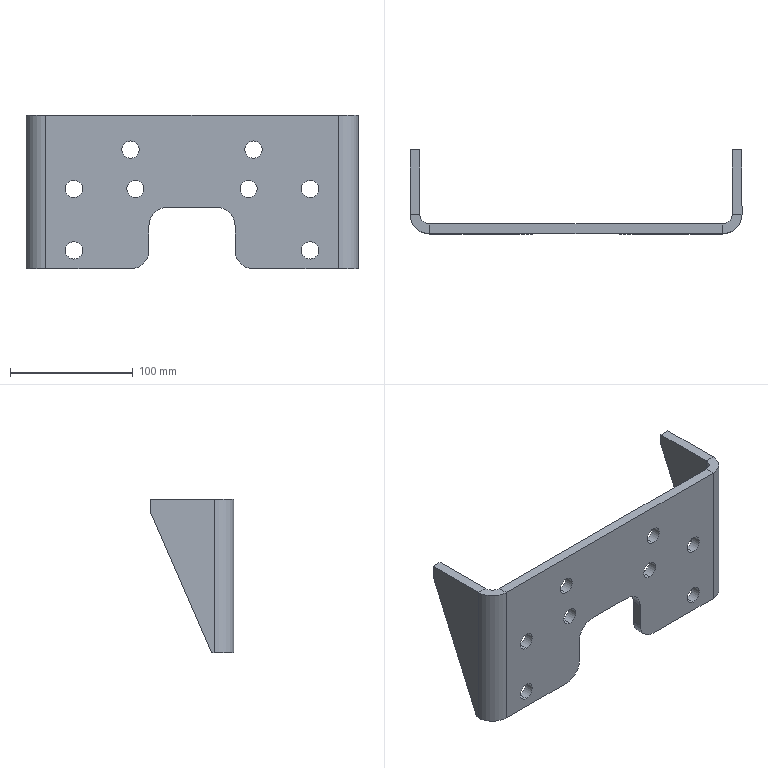Part | SolidWorks | features Extrusion 1, FlatPattern 1, SM3dBend 1, SheetMetal 1, SolidToSheetMetal 1 | 1 solid | 48 faces | box 270 x 68.15 x 125 mm | volume 296148 mm3 | cylinder 24 | plane 24 | commonest cylinder face diameters 14 x16 30 x4 16 x2 32 x2
STEP:
#1=CARTESIAN_POINT('',(96.,8.,-117.));
#2=VERTEX_POINT('',#1);
#3=CARTESIAN_POINT('',(96.,8.,-103.));
#4=VERTEX_POINT('',#3);
#5=CARTESIAN_POINT('',(96.,8.,-110.));
#6=DIRECTION('',(0.,1.,0.));
#7=DIRECTION('',(0.,0.,-1.));
#8=AXIS2_PLACEMENT_3D('',#5,#6,#7);
#9=CIRCLE('',#8,7.);
#10=EDGE_CURVE('',#2,#4,#9,.T.);
#11=ORIENTED_EDGE('',*,*,#10,.T.);
#12=CARTESIAN_POINT('',(96.,0.,-103.));
#13=VERTEX_POINT('',#12);
#14=CARTESIAN_POINT('',(96.,8.,-103.));
#15=DIRECTION('',(0.,-1.,0.));
#16=VECTOR('',#15,1000.);
#17=LINE('',#14,#16);
#18=EDGE_CURVE('',#4,#13,#17,.T.);
#19=ORIENTED_EDGE('',*,*,#18,.T.);
#20=CARTESIAN_POINT('',(96.,0.,-117.));
#21=VERTEX_POINT('',#20);
#22=CARTESIAN_POINT('',(96.,0.,-110.));
#23=DIRECTION('',(0.,1.,0.));
#24=DIRECTION('',(0.,0.,1.));
#25=AXIS2_PLACEMENT_3D('',#22,#23,#24);
#26=CIRCLE('',#25,7.);
#27=EDGE_CURVE('',#21,#13,#26,.T.);
#28=ORIENTED_EDGE('',*,*,#27,.F.);
#29=CARTESIAN_POINT('',(96.,8.,-117.));
#30=DIRECTION('',(0.,-1.,0.));
#31=VECTOR('',#30,1000.);
#32=LINE('',#29,#31);
#33=EDGE_CURVE('',#2,#21,#32,.T.);
#34=ORIENTED_EDGE('',*,*,#33,.F.);
#35=EDGE_LOOP('',(#11,#19,#28,#34));
#36=FACE_OUTER_BOUND('',#35,.T.);
#37=CARTESIAN_POINT('',(96.,8.,-110.));
#38=DIRECTION('',(0.,-1.,0.));
#39=DIRECTION('',(0.,0.,-1.));
#40=AXIS2_PLACEMENT_3D('',#37,#38,#39);
#41=CYLINDRICAL_SURFACE('',#40,7.);
#42=ADVANCED_FACE('',(#36),#41,.F.);
#43=CARTESIAN_POINT('',(96.,8.,-67.));
#44=VERTEX_POINT('',#43);
#45=CARTESIAN_POINT('',(96.,8.,-53.));
#46=VERTEX_POINT('',#45);
#47=CARTESIAN_POINT('',(96.,8.,-60.));
#48=DIRECTION('',(0.,1.,0.));
#49=DIRECTION('',(0.,0.,-1.));
#50=AXIS2_PLACEMENT_3D('',#47,#48,#49);
#51=CIRCLE('',#50,7.);
#52=EDGE_CURVE('',#44,#46,#51,.T.);
#53=ORIENTED_EDGE('',*,*,#52,.T.);
#54=CARTESIAN_POINT('',(96.,0.,-53.));
#55=VERTEX_POINT('',#54);
#56=CARTESIAN_POINT('',(96.,8.,-53.));
#57=DIRECTION('',(0.,-1.,0.));
#58=VECTOR('',#57,1000.);
#59=LINE('',#56,#58);
#60=EDGE_CURVE('',#46,#55,#59,.T.);
#61=ORIENTED_EDGE('',*,*,#60,.T.);
#62=CARTESIAN_POINT('',(96.,0.,-67.));
#63=VERTEX_POINT('',#62);
#64=CARTESIAN_POINT('',(96.,0.,-60.));
#65=DIRECTION('',(0.,1.,0.));
#66=DIRECTION('',(0.,0.,1.));
#67=AXIS2_PLACEMENT_3D('',#64,#65,#66);
#68=CIRCLE('',#67,7.);
#69=EDGE_CURVE('',#63,#55,#68,.T.);
#70=ORIENTED_EDGE('',*,*,#69,.F.);
#71=CARTESIAN_POINT('',(96.,8.,-67.));
#72=DIRECTION('',(0.,-1.,0.));
#73=VECTOR('',#72,1000.);
#74=LINE('',#71,#73);
#75=EDGE_CURVE('',#44,#63,#74,.T.);
#76=ORIENTED_EDGE('',*,*,#75,.F.);
#77=EDGE_LOOP('',(#53,#61,#70,#76));
#78=FACE_OUTER_BOUND('',#77,.T.);
#79=CARTESIAN_POINT('',(96.,8.,-60.));
#80=DIRECTION('',(0.,-1.,0.));
#81=DIRECTION('',(0.,0.,-1.));
#82=AXIS2_PLACEMENT_3D('',#79,#80,#81);
#83=CYLINDRICAL_SURFACE('',#82,7.);
#84=ADVANCED_FACE('',(#78),#83,.F.);
#85=CARTESIAN_POINT('',(46.,8.,-67.));
#86=VERTEX_POINT('',#85);
#87=CARTESIAN_POINT('',(46.,8.,-53.));
#88=VERTEX_POINT('',#87);
#89=CARTESIAN_POINT('',(46.,8.,-60.));
#90=DIRECTION('',(0.,1.,0.));
#91=DIRECTION('',(0.,0.,-1.));
#92=AXIS2_PLACEMENT_3D('',#89,#90,#91);
#93=CIRCLE('',#92,7.);
#94=EDGE_CURVE('',#86,#88,#93,.T.);
#95=ORIENTED_EDGE('',*,*,#94,.T.);
#96=CARTESIAN_POINT('',(46.,0.,-53.));
#97=VERTEX_POINT('',#96);
#98=CARTESIAN_POINT('',(46.,8.,-53.));
#99=DIRECTION('',(0.,-1.,0.));
#100=VECTOR('',#99,1000.);
#101=LINE('',#98,#100);
#102=EDGE_CURVE('',#88,#97,#101,.T.);
#103=ORIENTED_EDGE('',*,*,#102,.T.);
#104=CARTESIAN_POINT('',(46.,0.,-67.));
#105=VERTEX_POINT('',#104);
#106=CARTESIAN_POINT('',(46.,0.,-60.));
#107=DIRECTION('',(0.,1.,0.));
#108=DIRECTION('',(0.,0.,1.));
#109=AXIS2_PLACEMENT_3D('',#106,#107,#108);
#110=CIRCLE('',#109,7.);
#111=EDGE_CURVE('',#105,#97,#110,.T.);
#112=ORIENTED_EDGE('',*,*,#111,.F.);
#113=CARTESIAN_POINT('',(46.,8.,-67.));
#114=DIRECTION('',(0.,-1.,0.));
#115=VECTOR('',#114,1000.);
#116=LINE('',#113,#115);
#117=EDGE_CURVE('',#86,#105,#116,.T.);
#118=ORIENTED_EDGE('',*,*,#117,.F.);
#119=EDGE_LOOP('',(#95,#103,#112,#118));
#120=FACE_OUTER_BOUND('',#119,.T.);
#121=CARTESIAN_POINT('',(46.,8.,-60.));
#122=DIRECTION('',(0.,-1.,0.));
#123=DIRECTION('',(0.,0.,-1.));
#124=AXIS2_PLACEMENT_3D('',#121,#122,#123);
#125=CYLINDRICAL_SURFACE('',#124,7.);
#126=ADVANCED_FACE('',(#120),#125,.F.);
#127=CARTESIAN_POINT('',(50.,8.,-35.));
#128=VERTEX_POINT('',#127);
#129=CARTESIAN_POINT('',(50.,8.,-21.));
#130=VERTEX_POINT('',#129);
#131=CARTESIAN_POINT('',(50.,8.,-28.));
#132=DIRECTION('',(0.,1.,0.));
#133=DIRECTION('',(0.,0.,-1.));
#134=AXIS2_PLACEMENT_3D('',#131,#132,#133);
#135=CIRCLE('',#134,7.);
#136=EDGE_CURVE('',#128,#130,#135,.T.);
#137=ORIENTED_EDGE('',*,*,#136,.T.);
#138=CARTESIAN_POINT('',(50.,0.,-21.));
#139=VERTEX_POINT('',#138);
#140=CARTESIAN_POINT('',(50.,8.,-21.));
#141=DIRECTION('',(0.,-1.,0.));
#142=VECTOR('',#141,1000.);
#143=LINE('',#140,#142);
#144=EDGE_CURVE('',#130,#139,#143,.T.);
#145=ORIENTED_EDGE('',*,*,#144,.T.);
#146=CARTESIAN_POINT('',(50.,0.,-35.));
#147=VERTEX_POINT('',#146);
#148=CARTESIAN_POINT('',(50.,0.,-28.));
#149=DIRECTION('',(0.,1.,0.));
#150=DIRECTION('',(0.,0.,1.));
#151=AXIS2_PLACEMENT_3D('',#148,#149,#150);
#152=CIRCLE('',#151,7.);
#153=EDGE_CURVE('',#147,#139,#152,.T.);
#154=ORIENTED_EDGE('',*,*,#153,.F.);
#155=CARTESIAN_POINT('',(50.,8.,-35.));
#156=DIRECTION('',(0.,-1.,0.));
#157=VECTOR('',#156,1000.);
#158=LINE('',#155,#157);
#159=EDGE_CURVE('',#128,#147,#158,.T.);
#160=ORIENTED_EDGE('',*,*,#159,.F.);
#161=EDGE_LOOP('',(#137,#145,#154,#160));
#162=FACE_OUTER_BOUND('',#161,.T.);
#163=CARTESIAN_POINT('',(50.,8.,-28.));
#164=DIRECTION('',(0.,-1.,0.));
#165=DIRECTION('',(0.,0.,-1.));
#166=AXIS2_PLACEMENT_3D('',#163,#164,#165);
#167=CYLINDRICAL_SURFACE('',#166,7.);
#168=ADVANCED_FACE('',(#162),#167,.F.);
#169=CARTESIAN_POINT('',(-50.,8.,-35.));
#170=VERTEX_POINT('',#169);
#171=CARTESIAN_POINT('',(-50.,8.,-21.));
#172=VERTEX_POINT('',#171);
#173=CARTESIAN_POINT('',(-50.,8.,-28.));
#174=DIRECTION('',(0.,1.,0.));
#175=DIRECTION('',(0.,0.,1.));
#176=AXIS2_PLACEMENT_3D('',#173,#174,#175);
#177=CIRCLE('',#176,7.);
#178=EDGE_CURVE('',#170,#172,#177,.T.);
#179=ORIENTED_EDGE('',*,*,#178,.T.);
#180=CARTESIAN_POINT('',(-50.,0.,-21.));
#181=VERTEX_POINT('',#180);
#182=CARTESIAN_POINT('',(-50.,8.,-21.));
#183=DIRECTION('',(0.,-1.,0.));
#184=VECTOR('',#183,1000.);
#185=LINE('',#182,#184);
#186=EDGE_CURVE('',#172,#181,#185,.T.);
#187=ORIENTED_EDGE('',*,*,#186,.T.);
#188=CARTESIAN_POINT('',(-50.,0.,-35.));
#189=VERTEX_POINT('',#188);
#190=CARTESIAN_POINT('',(-50.,0.,-28.));
#191=DIRECTION('',(0.,1.,0.));
#192=DIRECTION('',(0.,0.,1.));
#193=AXIS2_PLACEMENT_3D('',#190,#191,#192);
#194=CIRCLE('',#193,7.);
#195=EDGE_CURVE('',#189,#181,#194,.T.);
#196=ORIENTED_EDGE('',*,*,#195,.F.);
#197=CARTESIAN_POINT('',(-50.,8.,-35.));
#198=DIRECTION('',(0.,-1.,0.));
#199=VECTOR('',#198,1000.);
#200=LINE('',#197,#199);
#201=EDGE_CURVE('',#170,#189,#200,.T.);
#202=ORIENTED_EDGE('',*,*,#201,.F.);
#203=EDGE_LOOP('',(#179,#187,#196,#202));
#204=FACE_OUTER_BOUND('',#203,.T.);
#205=CARTESIAN_POINT('',(-50.,8.,-28.));
#206=DIRECTION('',(0.,-1.,0.));
#207=DIRECTION('',(0.,0.,-1.));
#208=AXIS2_PLACEMENT_3D('',#205,#206,#207);
#209=CYLINDRICAL_SURFACE('',#208,7.);
#210=ADVANCED_FACE('',(#204),#209,.F.);
#211=CARTESIAN_POINT('',(-46.,8.,-67.));
#212=VERTEX_POINT('',#211);
#213=CARTESIAN_POINT('',(-46.,8.,-53.));
#214=VERTEX_POINT('',#213);
#215=CARTESIAN_POINT('',(-46.,8.,-60.));
#216=DIRECTION('',(0.,1.,0.));
#217=DIRECTION('',(0.,0.,1.));
#218=AXIS2_PLACEMENT_3D('',#215,#216,#217);
#219=CIRCLE('',#218,7.);
#220=EDGE_CURVE('',#212,#214,#219,.T.);
#221=ORIENTED_EDGE('',*,*,#220,.T.);
#222=CARTESIAN_POINT('',(-46.,0.,-53.));
#223=VERTEX_POINT('',#222);
#224=CARTESIAN_POINT('',(-46.,8.,-53.));
#225=DIRECTION('',(0.,-1.,0.));
#226=VECTOR('',#225,1000.);
#227=LINE('',#224,#226);
#228=EDGE_CURVE('',#214,#223,#227,.T.);
#229=ORIENTED_EDGE('',*,*,#228,.T.);
#230=CARTESIAN_POINT('',(-46.,0.,-67.));
#231=VERTEX_POINT('',#230);
#232=CARTESIAN_POINT('',(-46.,0.,-60.));
#233=DIRECTION('',(0.,1.,0.));
#234=DIRECTION('',(0.,0.,1.));
#235=AXIS2_PLACEMENT_3D('',#232,#233,#234);
#236=CIRCLE('',#235,7.);
#237=EDGE_CURVE('',#231,#223,#236,.T.);
#238=ORIENTED_EDGE('',*,*,#237,.F.);
#239=CARTESIAN_POINT('',(-46.,8.,-67.));
#240=DIRECTION('',(0.,-1.,0.));
#241=VECTOR('',#240,1000.);
#242=LINE('',#239,#241);
#243=EDGE_CURVE('',#212,#231,#242,.T.);
#244=ORIENTED_EDGE('',*,*,#243,.F.);
#245=EDGE_LOOP('',(#221,#229,#238,#244));
#246=FACE_OUTER_BOUND('',#245,.T.);
#247=CARTESIAN_POINT('',(-46.,8.,-60.));
#248=DIRECTION('',(0.,-1.,0.));
#249=DIRECTION('',(0.,0.,-1.));
#250=AXIS2_PLACEMENT_3D('',#247,#248,#249);
#251=CYLINDRICAL_SURFACE('',#250,7.);
#252=ADVANCED_FACE('',(#246),#251,.F.);
#253=CARTESIAN_POINT('',(-96.,8.,-67.));
#254=VERTEX_POINT('',#253);
#255=CARTESIAN_POINT('',(-96.,8.,-53.));
#256=VERTEX_POINT('',#255);
#257=CARTESIAN_POINT('',(-96.,8.,-60.));
#258=DIRECTION('',(0.,1.,0.));
#259=DIRECTION('',(0.,0.,1.));
#260=AXIS2_PLACEMENT_3D('',#257,#258,#259);
#261=CIRCLE('',#260,7.);
#262=EDGE_CURVE('',#254,#256,#261,.T.);
#263=ORIENTED_EDGE('',*,*,#262,.T.);
#264=CARTESIAN_POINT('',(-96.,0.,-53.));
#265=VERTEX_POINT('',#264);
#266=CARTESIAN_POINT('',(-96.,8.,-53.));
#267=DIRECTION('',(0.,-1.,0.));
#268=VECTOR('',#267,1000.);
#269=LINE('',#266,#268);
#270=EDGE_CURVE('',#256,#265,#269,.T.);
#271=ORIENTED_EDGE('',*,*,#270,.T.);
#272=CARTESIAN_POINT('',(-96.,0.,-67.));
#273=VERTEX_POINT('',#272);
#274=CARTESIAN_POINT('',(-96.,0.,-60.));
#275=DIRECTION('',(0.,1.,0.));
#276=DIRECTION('',(0.,0.,1.));
#277=AXIS2_PLACEMENT_3D('',#274,#275,#276);
#278=CIRCLE('',#277,7.);
#279=EDGE_CURVE('',#273,#265,#278,.T.);
#280=ORIENTED_EDGE('',*,*,#279,.F.);
#281=CARTESIAN_POINT('',(-96.,8.,-67.));
#282=DIRECTION('',(0.,-1.,0.));
#283=VECTOR('',#282,1000.);
#284=LINE('',#281,#283);
#285=EDGE_CURVE('',#254,#273,#284,.T.);
#286=ORIENTED_EDGE('',*,*,#285,.F.);
#287=EDGE_LOOP('',(#263,#271,#280,#286));
#288=FACE_OUTER_BOUND('',#287,.T.);
#289=CARTESIAN_POINT('',(-96.,8.,-60.));
#290=DIRECTION('',(0.,-1.,0.));
#291=DIRECTION('',(0.,0.,-1.));
#292=AXIS2_PLACEMENT_3D('',#289,#290,#291);
#293=CYLINDRICAL_SURFACE('',#292,7.);
#294=ADVANCED_FACE('',(#288),#293,.F.);
#295=CARTESIAN_POINT('',(-96.,8.,-117.));
#296=VERTEX_POINT('',#295);
#297=CARTESIAN_POINT('',(-96.,8.,-103.));
#298=VERTEX_POINT('',#297);
#299=CARTESIAN_POINT('',(-96.,8.,-110.));
#300=DIRECTION('',(0.,1.,0.));
#301=DIRECTION('',(0.,0.,1.));
#302=AXIS2_PLACEMENT_3D('',#299,#300,#301);
#303=CIRCLE('',#302,7.);
#304=EDGE_CURVE('',#296,#298,#303,.T.);
#305=ORIENTED_EDGE('',*,*,#304,.T.);
#306=CARTESIAN_POINT('',(-96.,0.,-103.));
#307=VERTEX_POINT('',#306);
#308=CARTESIAN_POINT('',(-96.,8.,-103.));
#309=DIRECTION('',(0.,-1.,0.));
#310=VECTOR('',#309,1000.);
#311=LINE('',#308,#310);
#312=EDGE_CURVE('',#298,#307,#311,.T.);
#313=ORIENTED_EDGE('',*,*,#312,.T.);
#314=CARTESIAN_POINT('',(-96.,0.,-117.));
#315=VERTEX_POINT('',#314);
#316=CARTESIAN_POINT('',(-96.,0.,-110.));
#317=DIRECTION('',(0.,1.,0.));
#318=DIRECTION('',(0.,0.,1.));
#319=AXIS2_PLACEMENT_3D('',#316,#317,#318);
#320=CIRCLE('',#319,7.);
#321=EDGE_CURVE('',#315,#307,#320,.T.);
#322=ORIENTED_EDGE('',*,*,#321,.F.);
#323=CARTESIAN_POINT('',(-96.,8.,-117.));
#324=DIRECTION('',(0.,-1.,0.));
#325=VECTOR('',#324,1000.);
#326=LINE('',#323,#325);
#327=EDGE_CURVE('',#296,#315,#326,.T.);
#328=ORIENTED_EDGE('',*,*,#327,.F.);
#329=EDGE_LOOP('',(#305,#313,#322,#328));
#330=FACE_OUTER_BOUND('',#329,.T.);
#331=CARTESIAN_POINT('',(-96.,8.,-110.));
#332=DIRECTION('',(0.,-1.,0.));
#333=DIRECTION('',(0.,0.,-1.));
#334=AXIS2_PLACEMENT_3D('',#331,#332,#333);
#335=CYLINDRICAL_SURFACE('',#334,7.);
#336=ADVANCED_FACE('',(#330),#335,.F.);
#337=ORIENTED_EDGE('',*,*,#321,.T.);
#338=CARTESIAN_POINT('',(-96.,0.,-110.));
#339=DIRECTION('',(0.,1.,0.));
#340=DIRECTION('',(0.,0.,1.));
#341=AXIS2_PLACEMENT_3D('',#338,#339,#340);
#342=CIRCLE('',#341,7.);
#343=EDGE_CURVE('',#307,#315,#342,.T.);
#344=ORIENTED_EDGE('',*,*,#343,.T.);
#345=EDGE_LOOP('',(#337,#344));
#346=FACE_BOUND('',#345,.T.);
#347=ORIENTED_EDGE('',*,*,#279,.T.);
#348=CARTESIAN_POINT('',(-96.,0.,-60.));
#349=DIRECTION('',(0.,1.,0.));
#350=DIRECTION('',(0.,0.,1.));
#351=AXIS2_PLACEMENT_3D('',#348,#349,#350);
#352=CIRCLE('',#351,7.);
#353=EDGE_CURVE('',#265,#273,#352,.T.);
#354=ORIENTED_EDGE('',*,*,#353,.T.);
#355=EDGE_LOOP('',(#347,#354));
#356=FACE_BOUND('',#355,.T.);
#357=ORIENTED_EDGE('',*,*,#237,.T.);
#358=CARTESIAN_POINT('',(-46.,0.,-60.));
#359=DIRECTION('',(0.,1.,0.));
#360=DIRECTION('',(0.,0.,1.));
#361=AXIS2_PLACEMENT_3D('',#358,#359,#360);
#362=CIRCLE('',#361,7.);
#363=EDGE_CURVE('',#223,#231,#362,.T.);
#364=ORIENTED_EDGE('',*,*,#363,.T.);
#365=EDGE_LOOP('',(#357,#364));
#366=FACE_BOUND('',#365,.T.);
#367=ORIENTED_EDGE('',*,*,#195,.T.);
#368=CARTESIAN_POINT('',(-50.,0.,-28.));
#369=DIRECTION('',(0.,1.,0.));
#370=DIRECTION('',(0.,0.,1.));
#371=AXIS2_PLACEMENT_3D('',#368,#369,#370);
#372=CIRCLE('',#371,7.);
#373=EDGE_CURVE('',#181,#189,#372,.T.);
#374=ORIENTED_EDGE('',*,*,#373,.T.);
#375=EDGE_LOOP('',(#367,#374));
#376=FACE_BOUND('',#375,.T.);
#377=ORIENTED_EDGE('',*,*,#153,.T.);
#378=CARTESIAN_POINT('',(50.,0.,-28.));
#379=DIRECTION('',(0.,1.,0.));
#380=DIRECTION('',(0.,0.,1.));
#381=AXIS2_PLACEMENT_3D('',#378,#379,#380);
#382=CIRCLE('',#381,7.);
#383=EDGE_CURVE('',#139,#147,#382,.T.);
#384=ORIENTED_EDGE('',*,*,#383,.T.);
#385=EDGE_LOOP('',(#377,#384));
#386=FACE_BOUND('',#385,.T.);
#387=ORIENTED_EDGE('',*,*,#111,.T.);
#388=CARTESIAN_POINT('',(46.,0.,-60.));
#389=DIRECTION('',(0.,1.,0.));
#390=DIRECTION('',(0.,0.,1.));
#391=AXIS2_PLACEMENT_3D('',#388,#389,#390);
#392=CIRCLE('',#391,7.);
#393=EDGE_CURVE('',#97,#105,#392,.T.);
#394=ORIENTED_EDGE('',*,*,#393,.T.);
#395=EDGE_LOOP('',(#387,#394));
#396=FACE_BOUND('',#395,.T.);
#397=ORIENTED_EDGE('',*,*,#69,.T.);
#398=CARTESIAN_POINT('',(96.,0.,-60.));
#399=DIRECTION('',(0.,1.,0.));
#400=DIRECTION('',(0.,0.,1.));
#401=AXIS2_PLACEMENT_3D('',#398,#399,#400);
#402=CIRCLE('',#401,7.);
#403=EDGE_CURVE('',#55,#63,#402,.T.);
#404=ORIENTED_EDGE('',*,*,#403,.T.);
#405=EDGE_LOOP('',(#397,#404));
#406=FACE_BOUND('',#405,.T.);
#407=ORIENTED_EDGE('',*,*,#27,.T.);
#408=CARTESIAN_POINT('',(96.,0.,-110.));
#409=DIRECTION('',(0.,1.,0.));
#410=DIRECTION('',(0.,0.,1.));
#411=AXIS2_PLACEMENT_3D('',#408,#409,#410);
#412=CIRCLE('',#411,7.);
#413=EDGE_CURVE('',#13,#21,#412,.T.);
#414=ORIENTED_EDGE('',*,*,#413,.T.);
#415=EDGE_LOOP('',(#407,#414));
#416=FACE_BOUND('',#415,.T.);
#417=CARTESIAN_POINT('',(119.,0.,-125.));
#418=VERTEX_POINT('',#417);
#419=CARTESIAN_POINT('',(50.,0.,-125.));
#420=VERTEX_POINT('',#419);
#421=CARTESIAN_POINT('',(-50.,0.,-125.));
#422=DIRECTION('',(-1.,0.,0.));
#423=VECTOR('',#422,1000.);
#424=LINE('',#421,#423);
#425=EDGE_CURVE('',#418,#420,#424,.T.);
#426=ORIENTED_EDGE('',*,*,#425,.F.);
#427=CARTESIAN_POINT('',(119.,0.,0.));
#428=VERTEX_POINT('',#427);
#429=CARTESIAN_POINT('',(119.,0.,-110.));
#430=DIRECTION('',(0.,0.,1.));
#431=VECTOR('',#430,1000.);
#432=LINE('',#429,#431);
#433=EDGE_CURVE('',#418,#428,#432,.T.);
#434=ORIENTED_EDGE('',*,*,#433,.T.);
#435=CARTESIAN_POINT('',(-119.,0.,0.));
#436=VERTEX_POINT('',#435);
#437=CARTESIAN_POINT('',(-50.,0.,0.));
#438=DIRECTION('',(1.,0.,0.));
#439=VECTOR('',#438,1000.);
#440=LINE('',#437,#439);
#441=EDGE_CURVE('',#436,#428,#440,.T.);
#442=ORIENTED_EDGE('',*,*,#441,.F.);
#443=CARTESIAN_POINT('',(-119.,0.,-125.));
#444=VERTEX_POINT('',#443);
#445=CARTESIAN_POINT('',(-119.,0.,-110.));
#446=DIRECTION('',(0.,0.,1.));
#447=VECTOR('',#446,1000.);
#448=LINE('',#445,#447);
#449=EDGE_CURVE('',#444,#436,#448,.T.);
#450=ORIENTED_EDGE('',*,*,#449,.F.);
#451=CARTESIAN_POINT('',(-50.,0.,-125.));
#452=VERTEX_POINT('',#451);
#453=CARTESIAN_POINT('',(-50.,0.,-125.));
#454=DIRECTION('',(-1.,0.,0.));
#455=VECTOR('',#454,1000.);
#456=LINE('',#453,#455);
#457=EDGE_CURVE('',#452,#444,#456,.T.);
#458=ORIENTED_EDGE('',*,*,#457,.F.);
#459=CARTESIAN_POINT('',(-35.,0.,-110.));
#460=VERTEX_POINT('',#459);
#461=CARTESIAN_POINT('',(-50.,0.,-110.));
#462=DIRECTION('',(0.,1.,0.));
#463=DIRECTION('',(0.,0.,1.));
#464=AXIS2_PLACEMENT_3D('',#461,#462,#463);
#465=CIRCLE('',#464,15.);
#466=EDGE_CURVE('',#460,#452,#465,.T.);
#467=ORIENTED_EDGE('',*,*,#466,.F.);
#468=CARTESIAN_POINT('',(-35.,0.,-90.));
#469=VERTEX_POINT('',#468);
#470=CARTESIAN_POINT('',(-35.,0.,-110.));
#471=DIRECTION('',(0.,0.,-1.));
#472=VECTOR('',#471,1000.);
#473=LINE('',#470,#472);
#474=EDGE_CURVE('',#469,#460,#473,.T.);
#475=ORIENTED_EDGE('',*,*,#474,.F.);
#476=CARTESIAN_POINT('',(-20.,0.,-75.));
#477=VERTEX_POINT('',#476);
#478=CARTESIAN_POINT('',(-20.,0.,-90.));
#479=DIRECTION('',(0.,-1.,0.));
#480=DIRECTION('',(0.,0.,-1.));
#481=AXIS2_PLACEMENT_3D('',#478,#479,#480);
#482=CIRCLE('',#481,15.);
#483=EDGE_CURVE('',#477,#469,#482,.T.);
#484=ORIENTED_EDGE('',*,*,#483,.F.);
#485=CARTESIAN_POINT('',(20.,0.,-75.));
#486=VERTEX_POINT('',#485);
#487=CARTESIAN_POINT('',(-50.,0.,-75.));
#488=DIRECTION('',(-1.,0.,0.));
#489=VECTOR('',#488,1000.);
#490=LINE('',#487,#489);
#491=EDGE_CURVE('',#486,#477,#490,.T.);
#492=ORIENTED_EDGE('',*,*,#491,.F.);
#493=CARTESIAN_POINT('',(35.,0.,-90.));
#494=VERTEX_POINT('',#493);
#495=CARTESIAN_POINT('',(20.,0.,-90.));
#496=DIRECTION('',(0.,-1.,0.));
#497=DIRECTION('',(0.,0.,-1.));
#498=AXIS2_PLACEMENT_3D('',#495,#496,#497);
#499=CIRCLE('',#498,15.);
#500=EDGE_CURVE('',#494,#486,#499,.T.);
#501=ORIENTED_EDGE('',*,*,#500,.F.);
#502=CARTESIAN_POINT('',(35.,0.,-110.));
#503=VERTEX_POINT('',#502);
#504=CARTESIAN_POINT('',(35.,0.,-110.));
#505=DIRECTION('',(0.,0.,1.));
#506=VECTOR('',#505,1000.);
#507=LINE('',#504,#506);
#508=EDGE_CURVE('',#503,#494,#507,.T.);
#509=ORIENTED_EDGE('',*,*,#508,.F.);
#510=CARTESIAN_POINT('',(50.,0.,-110.));
#511=DIRECTION('',(0.,1.,0.));
#512=DIRECTION('',(0.,0.,1.));
#513=AXIS2_PLACEMENT_3D('',#510,#511,#512);
#514=CIRCLE('',#513,15.);
#515=EDGE_CURVE('',#420,#503,#514,.T.);
#516=ORIENTED_EDGE('',*,*,#515,.F.);
#517=EDGE_LOOP('',(#426,#434,#442,#450,#458,#467,#475,#484,#492,#501,#509,#516));
#518=FACE_OUTER_BOUND('',#517,.T.);
#519=CARTESIAN_POINT('',(-50.,0.,-110.));
#520=DIRECTION('',(0.,-1.,0.));
#521=DIRECTION('',(0.,0.,-1.));
#522=AXIS2_PLACEMENT_3D('',#519,#520,#521);
#523=PLANE('',#522);
#524=ADVANCED_FACE('',(#346,#356,#366,#376,#386,#396,#406,#416,#518),#523,.T.);
#525=ORIENTED_EDGE('',*,*,#441,.T.);
#526=CARTESIAN_POINT('',(119.,8.,0.));
#527=VERTEX_POINT('',#526);
#528=CARTESIAN_POINT('',(119.,8.,0.));
#529=DIRECTION('',(0.,1.,0.));
#530=VECTOR('',#529,1000.);
#531=LINE('',#528,#530);
#532=EDGE_CURVE('',#428,#527,#531,.T.);
#533=ORIENTED_EDGE('',*,*,#532,.T.);
#534=CARTESIAN_POINT('',(-119.,8.,0.));
#535=VERTEX_POINT('',#534);
#536=CARTESIAN_POINT('',(-190.,8.,0.));
#537=DIRECTION('',(1.,0.,0.));
#538=VECTOR('',#537,1000.);
#539=LINE('',#536,#538);
#540=EDGE_CURVE('',#535,#527,#539,.T.);
#541=ORIENTED_EDGE('',*,*,#540,.F.);
#542=CARTESIAN_POINT('',(-119.,8.,0.));
#543=DIRECTION('',(0.,1.,0.));
#544=VECTOR('',#543,1000.);
#545=LINE('',#542,#544);
#546=EDGE_CURVE('',#436,#535,#545,.T.);
#547=ORIENTED_EDGE('',*,*,#546,.F.);
#548=EDGE_LOOP('',(#525,#533,#541,#547));
#549=FACE_OUTER_BOUND('',#548,.T.);
#550=CARTESIAN_POINT('',(-190.,8.,0.));
#551=DIRECTION('',(0.,0.,-1.));
#552=DIRECTION('',(1.,0.,0.));
#553=AXIS2_PLACEMENT_3D('',#550,#551,#552);
#554=PLANE('',#553);
#555=ADVANCED_FACE('',(#549),#554,.F.);
#556=CARTESIAN_POINT('',(119.,8.,-125.));
#557=VERTEX_POINT('',#556);
#558=CARTESIAN_POINT('',(50.,8.,-125.));
#559=VERTEX_POINT('',#558);
#560=CARTESIAN_POINT('',(140.,8.,-125.));
#561=DIRECTION('',(-1.,0.,0.));
#562=VECTOR('',#561,1000.);
#563=LINE('',#560,#562);
#564=EDGE_CURVE('',#557,#559,#563,.T.);
#565=ORIENTED_EDGE('',*,*,#564,.F.);
#566=CARTESIAN_POINT('',(119.,8.,-125.));
#567=DIRECTION('',(0.,-1.,0.));
#568=VECTOR('',#567,1000.);
#569=LINE('',#566,#568);
#570=EDGE_CURVE('',#557,#418,#569,.T.);
#571=ORIENTED_EDGE('',*,*,#570,.T.);
#572=ORIENTED_EDGE('',*,*,#425,.T.);
#573=CARTESIAN_POINT('',(50.,8.,-125.));
#574=DIRECTION('',(0.,1.,0.));
#575=VECTOR('',#574,1000.);
#576=LINE('',#573,#575);
#577=EDGE_CURVE('',#420,#559,#576,.T.);
#578=ORIENTED_EDGE('',*,*,#577,.T.);
#579=EDGE_LOOP('',(#565,#571,#572,#578));
#580=FACE_OUTER_BOUND('',#579,.T.);
#581=CARTESIAN_POINT('',(140.,8.,-125.));
#582=DIRECTION('',(0.,0.,1.));
#583=DIRECTION('',(-1.,0.,0.));
#584=AXIS2_PLACEMENT_3D('',#581,#582,#583);
#585=PLANE('',#584);
#586=ADVANCED_FACE('',(#580),#585,.F.);
#587=CARTESIAN_POINT('',(119.,8.,-110.));
#588=DIRECTION('',(0.,0.,1.));
#589=VECTOR('',#588,1000.);
#590=LINE('',#587,#589);
#591=EDGE_CURVE('',#557,#527,#590,.T.);
#592=ORIENTED_EDGE('',*,*,#591,.F.);
#593=ORIENTED_EDGE('',*,*,#564,.T.);
#594=CARTESIAN_POINT('',(35.,8.,-110.));
#595=VERTEX_POINT('',#594);
#596=CARTESIAN_POINT('',(50.,8.,-110.));
#597=DIRECTION('',(0.,1.,0.));
#598=DIRECTION('',(0.,0.,1.));
#599=AXIS2_PLACEMENT_3D('',#596,#597,#598);
#600=CIRCLE('',#599,15.);
#601=EDGE_CURVE('',#559,#595,#600,.T.);
#602=ORIENTED_EDGE('',*,*,#601,.T.);
#603=CARTESIAN_POINT('',(35.,8.,-90.));
#604=VERTEX_POINT('',#603);
#605=CARTESIAN_POINT('',(35.,8.,-110.));
#606=DIRECTION('',(0.,0.,1.));
#607=VECTOR('',#606,1000.);
#608=LINE('',#605,#607);
#609=EDGE_CURVE('',#595,#604,#608,.T.);
#610=ORIENTED_EDGE('',*,*,#609,.T.);
#611=CARTESIAN_POINT('',(20.,8.,-75.));
#612=VERTEX_POINT('',#611);
#613=CARTESIAN_POINT('',(20.,8.,-90.));
#614=DIRECTION('',(0.,-1.,0.));
#615=DIRECTION('',(0.,0.,-1.));
#616=AXIS2_PLACEMENT_3D('',#613,#614,#615);
#617=CIRCLE('',#616,15.);
#618=EDGE_CURVE('',#604,#612,#617,.T.);
#619=ORIENTED_EDGE('',*,*,#618,.T.);
#620=CARTESIAN_POINT('',(-20.,8.,-75.));
#621=VERTEX_POINT('',#620);
#622=CARTESIAN_POINT('',(-20.,8.,-75.));
#623=DIRECTION('',(-1.,0.,0.));
#624=VECTOR('',#623,1000.);
#625=LINE('',#622,#624);
#626=EDGE_CURVE('',#612,#621,#625,.T.);
#627=ORIENTED_EDGE('',*,*,#626,.T.);
#628=CARTESIAN_POINT('',(-35.,8.,-90.));
#629=VERTEX_POINT('',#628);
#630=CARTESIAN_POINT('',(-20.,8.,-90.));
#631=DIRECTION('',(0.,-1.,0.));
#632=DIRECTION('',(0.,0.,1.));
#633=AXIS2_PLACEMENT_3D('',#630,#631,#632);
#634=CIRCLE('',#633,15.);
#635=EDGE_CURVE('',#621,#629,#634,.T.);
#636=ORIENTED_EDGE('',*,*,#635,.T.);
#637=CARTESIAN_POINT('',(-35.,8.,-110.));
#638=VERTEX_POINT('',#637);
#639=CARTESIAN_POINT('',(-35.,8.,-110.));
#640=DIRECTION('',(0.,0.,-1.));
#641=VECTOR('',#640,1000.);
#642=LINE('',#639,#641);
#643=EDGE_CURVE('',#629,#638,#642,.T.);
#644=ORIENTED_EDGE('',*,*,#643,.T.);
#645=CARTESIAN_POINT('',(-50.,8.,-125.));
#646=VERTEX_POINT('',#645);
#647=CARTESIAN_POINT('',(-50.,8.,-110.));
#648=DIRECTION('',(0.,1.,0.));
#649=DIRECTION('',(0.,0.,-1.));
#650=AXIS2_PLACEMENT_3D('',#647,#648,#649);
#651=CIRCLE('',#650,15.);
#652=EDGE_CURVE('',#638,#646,#651,.T.);
#653=ORIENTED_EDGE('',*,*,#652,.T.);
#654=CARTESIAN_POINT('',(-119.,8.,-125.));
#655=VERTEX_POINT('',#654);
#656=CARTESIAN_POINT('',(-140.,8.,-125.));
#657=DIRECTION('',(-1.,0.,0.));
#658=VECTOR('',#657,1000.);
#659=LINE('',#656,#658);
#660=EDGE_CURVE('',#646,#655,#659,.T.);
#661=ORIENTED_EDGE('',*,*,#660,.T.);
#662=CARTESIAN_POINT('',(-119.,8.,-110.));
#663=DIRECTION('',(0.,0.,1.));
#664=VECTOR('',#663,1000.);
#665=LINE('',#662,#664);
#666=EDGE_CURVE('',#655,#535,#665,.T.);
#667=ORIENTED_EDGE('',*,*,#666,.T.);
#668=ORIENTED_EDGE('',*,*,#540,.T.);
#669=EDGE_LOOP('',(#592,#593,#602,#610,#619,#627,#636,#644,#653,#661,#667,#668));
#670=FACE_OUTER_BOUND('',#669,.T.);
#671=ORIENTED_EDGE('',*,*,#304,.F.);
#672=CARTESIAN_POINT('',(-96.,8.,-110.));
#673=DIRECTION('',(0.,1.,0.));
#674=DIRECTION('',(0.,0.,1.));
#675=AXIS2_PLACEMENT_3D('',#672,#673,#674);
#676=CIRCLE('',#675,7.);
#677=EDGE_CURVE('',#298,#296,#676,.T.);
#678=ORIENTED_EDGE('',*,*,#677,.F.);
#679=EDGE_LOOP('',(#671,#678));
#680=FACE_BOUND('',#679,.T.);
#681=ORIENTED_EDGE('',*,*,#262,.F.);
#682=CARTESIAN_POINT('',(-96.,8.,-60.));
#683=DIRECTION('',(0.,1.,0.));
#684=DIRECTION('',(0.,0.,1.));
#685=AXIS2_PLACEMENT_3D('',#682,#683,#684);
#686=CIRCLE('',#685,7.);
#687=EDGE_CURVE('',#256,#254,#686,.T.);
#688=ORIENTED_EDGE('',*,*,#687,.F.);
#689=EDGE_LOOP('',(#681,#688));
#690=FACE_BOUND('',#689,.T.);
#691=ORIENTED_EDGE('',*,*,#220,.F.);
#692=CARTESIAN_POINT('',(-46.,8.,-60.));
#693=DIRECTION('',(0.,1.,0.));
#694=DIRECTION('',(0.,0.,1.));
#695=AXIS2_PLACEMENT_3D('',#692,#693,#694);
#696=CIRCLE('',#695,7.);
#697=EDGE_CURVE('',#214,#212,#696,.T.);
#698=ORIENTED_EDGE('',*,*,#697,.F.);
#699=EDGE_LOOP('',(#691,#698));
#700=FACE_BOUND('',#699,.T.);
#701=ORIENTED_EDGE('',*,*,#178,.F.);
#702=CARTESIAN_POINT('',(-50.,8.,-28.));
#703=DIRECTION('',(0.,1.,0.));
#704=DIRECTION('',(0.,0.,1.));
#705=AXIS2_PLACEMENT_3D('',#702,#703,#704);
#706=CIRCLE('',#705,7.);
#707=EDGE_CURVE('',#172,#170,#706,.T.);
#708=ORIENTED_EDGE('',*,*,#707,.F.);
#709=EDGE_LOOP('',(#701,#708));
#710=FACE_BOUND('',#709,.T.);
#711=ORIENTED_EDGE('',*,*,#136,.F.);
#712=CARTESIAN_POINT('',(50.,8.,-28.));
#713=DIRECTION('',(0.,1.,0.));
#714=DIRECTION('',(0.,0.,-1.));
#715=AXIS2_PLACEMENT_3D('',#712,#713,#714);
#716=CIRCLE('',#715,7.);
#717=EDGE_CURVE('',#130,#128,#716,.T.);
#718=ORIENTED_EDGE('',*,*,#717,.F.);
#719=EDGE_LOOP('',(#711,#718));
#720=FACE_BOUND('',#719,.T.);
#721=ORIENTED_EDGE('',*,*,#94,.F.);
#722=CARTESIAN_POINT('',(46.,8.,-60.));
#723=DIRECTION('',(0.,1.,0.));
#724=DIRECTION('',(0.,0.,-1.));
#725=AXIS2_PLACEMENT_3D('',#722,#723,#724);
#726=CIRCLE('',#725,7.);
#727=EDGE_CURVE('',#88,#86,#726,.T.);
#728=ORIENTED_EDGE('',*,*,#727,.F.);
#729=EDGE_LOOP('',(#721,#728));
#730=FACE_BOUND('',#729,.T.);
#731=ORIENTED_EDGE('',*,*,#52,.F.);
#732=CARTESIAN_POINT('',(96.,8.,-60.));
#733=DIRECTION('',(0.,1.,0.));
#734=DIRECTION('',(0.,0.,-1.));
#735=AXIS2_PLACEMENT_3D('',#732,#733,#734);
#736=CIRCLE('',#735,7.);
#737=EDGE_CURVE('',#46,#44,#736,.T.);
#738=ORIENTED_EDGE('',*,*,#737,.F.);
#739=EDGE_LOOP('',(#731,#738));
#740=FACE_BOUND('',#739,.T.);
#741=ORIENTED_EDGE('',*,*,#10,.F.);
#742=CARTESIAN_POINT('',(96.,8.,-110.));
#743=DIRECTION('',(0.,1.,0.));
#744=DIRECTION('',(0.,0.,-1.));
#745=AXIS2_PLACEMENT_3D('',#742,#743,#744);
#746=CIRCLE('',#745,7.);
#747=EDGE_CURVE('',#4,#2,#746,.T.);
#748=ORIENTED_EDGE('',*,*,#747,.F.);
#749=EDGE_LOOP('',(#741,#748));
#750=FACE_BOUND('',#749,.T.);
#751=CARTESIAN_POINT('',(-50.,8.,-110.));
#752=DIRECTION('',(0.,-1.,0.));
#753=DIRECTION('',(0.,0.,-1.));
#754=AXIS2_PLACEMENT_3D('',#751,#752,#753);
#755=PLANE('',#754);
#756=ADVANCED_FACE('',(#670,#680,#690,#700,#710,#720,#730,#740,#750),#755,.F.);
#757=ORIENTED_EDGE('',*,*,#577,.F.);
#758=ORIENTED_EDGE('',*,*,#515,.T.);
#759=CARTESIAN_POINT('',(35.,8.,-110.));
#760=DIRECTION('',(0.,1.,0.));
#761=VECTOR('',#760,1000.);
#762=LINE('',#759,#761);
#763=EDGE_CURVE('',#503,#595,#762,.T.);
#764=ORIENTED_EDGE('',*,*,#763,.T.);
#765=ORIENTED_EDGE('',*,*,#601,.F.);
#766=EDGE_LOOP('',(#757,#758,#764,#765));
#767=FACE_OUTER_BOUND('',#766,.T.);
#768=CARTESIAN_POINT('',(50.,8.,-110.));
#769=DIRECTION('',(0.,-1.,0.));
#770=DIRECTION('',(0.,0.,-1.));
#771=AXIS2_PLACEMENT_3D('',#768,#769,#770);
#772=CYLINDRICAL_SURFACE('',#771,15.);
#773=ADVANCED_FACE('',(#767),#772,.T.);
#774=ORIENTED_EDGE('',*,*,#763,.F.);
#775=ORIENTED_EDGE('',*,*,#508,.T.);
#776=CARTESIAN_POINT('',(35.,8.,-90.));
#777=DIRECTION('',(0.,1.,0.));
#778=VECTOR('',#777,1000.);
#779=LINE('',#776,#778);
#780=EDGE_CURVE('',#494,#604,#779,.T.);
#781=ORIENTED_EDGE('',*,*,#780,.T.);
#782=ORIENTED_EDGE('',*,*,#609,.F.);
#783=EDGE_LOOP('',(#774,#775,#781,#782));
#784=FACE_OUTER_BOUND('',#783,.T.);
#785=CARTESIAN_POINT('',(35.,8.,-110.));
#786=DIRECTION('',(1.,0.,0.));
#787=DIRECTION('',(0.,0.,1.));
#788=AXIS2_PLACEMENT_3D('',#785,#786,#787);
#789=PLANE('',#788);
#790=ADVANCED_FACE('',(#784),#789,.F.);
#791=ORIENTED_EDGE('',*,*,#780,.F.);
#792=ORIENTED_EDGE('',*,*,#500,.T.);
#793=CARTESIAN_POINT('',(20.,8.,-75.));
#794=DIRECTION('',(0.,1.,0.));
#795=VECTOR('',#794,1000.);
#796=LINE('',#793,#795);
#797=EDGE_CURVE('',#486,#612,#796,.T.);
#798=ORIENTED_EDGE('',*,*,#797,.T.);
#799=ORIENTED_EDGE('',*,*,#618,.F.);
#800=EDGE_LOOP('',(#791,#792,#798,#799));
#801=FACE_OUTER_BOUND('',#800,.T.);
#802=CARTESIAN_POINT('',(20.,8.,-90.));
#803=DIRECTION('',(0.,-1.,0.));
#804=DIRECTION('',(0.,0.,-1.));
#805=AXIS2_PLACEMENT_3D('',#802,#803,#804);
#806=CYLINDRICAL_SURFACE('',#805,15.);
#807=ADVANCED_FACE('',(#801),#806,.F.);
#808=ORIENTED_EDGE('',*,*,#797,.F.);
#809=ORIENTED_EDGE('',*,*,#491,.T.);
#810=CARTESIAN_POINT('',(-20.,8.,-75.));
#811=DIRECTION('',(0.,1.,0.));
#812=VECTOR('',#811,1000.);
#813=LINE('',#810,#812);
#814=EDGE_CURVE('',#477,#621,#813,.T.);
#815=ORIENTED_EDGE('',*,*,#814,.T.);
#816=ORIENTED_EDGE('',*,*,#626,.F.);
#817=EDGE_LOOP('',(#808,#809,#815,#816));
#818=FACE_OUTER_BOUND('',#817,.T.);
#819=CARTESIAN_POINT('',(-20.,8.,-75.));
#820=DIRECTION('',(0.,0.,1.));
#821=DIRECTION('',(-1.,0.,0.));
#822=AXIS2_PLACEMENT_3D('',#819,#820,#821);
#823=PLANE('',#822);
#824=ADVANCED_FACE('',(#818),#823,.F.);
#825=ORIENTED_EDGE('',*,*,#814,.F.);
#826=ORIENTED_EDGE('',*,*,#483,.T.);
#827=CARTESIAN_POINT('',(-35.,8.,-90.));
#828=DIRECTION('',(0.,1.,0.));
#829=VECTOR('',#828,1000.);
#830=LINE('',#827,#829);
#831=EDGE_CURVE('',#469,#629,#830,.T.);
#832=ORIENTED_EDGE('',*,*,#831,.T.);
#833=ORIENTED_EDGE('',*,*,#635,.F.);
#834=EDGE_LOOP('',(#825,#826,#832,#833));
#835=FACE_OUTER_BOUND('',#834,.T.);
#836=CARTESIAN_POINT('',(-20.,8.,-90.));
#837=DIRECTION('',(0.,-1.,0.));
#838=DIRECTION('',(0.,0.,-1.));
#839=AXIS2_PLACEMENT_3D('',#836,#837,#838);
#840=CYLINDRICAL_SURFACE('',#839,15.);
#841=ADVANCED_FACE('',(#835),#840,.F.);
#842=ORIENTED_EDGE('',*,*,#831,.F.);
#843=ORIENTED_EDGE('',*,*,#474,.T.);
#844=CARTESIAN_POINT('',(-35.,8.,-110.));
#845=DIRECTION('',(0.,1.,0.));
#846=VECTOR('',#845,1000.);
#847=LINE('',#844,#846);
#848=EDGE_CURVE('',#460,#638,#847,.T.);
#849=ORIENTED_EDGE('',*,*,#848,.T.);
#850=ORIENTED_EDGE('',*,*,#643,.F.);
#851=EDGE_LOOP('',(#842,#843,#849,#850));
#852=FACE_OUTER_BOUND('',#851,.T.);
#853=CARTESIAN_POINT('',(-35.,8.,-110.));
#854=DIRECTION('',(-1.,0.,0.));
#855=DIRECTION('',(0.,0.,-1.));
#856=AXIS2_PLACEMENT_3D('',#853,#854,#855);
#857=PLANE('',#856);
#858=ADVANCED_FACE('',(#852),#857,.F.);
#859=ORIENTED_EDGE('',*,*,#848,.F.);
#860=ORIENTED_EDGE('',*,*,#466,.T.);
#861=CARTESIAN_POINT('',(-50.,8.,-125.));
#862=DIRECTION('',(0.,1.,0.));
#863=VECTOR('',#862,1000.);
#864=LINE('',#861,#863);
#865=EDGE_CURVE('',#452,#646,#864,.T.);
#866=ORIENTED_EDGE('',*,*,#865,.T.);
#867=ORIENTED_EDGE('',*,*,#652,.F.);
#868=EDGE_LOOP('',(#859,#860,#866,#867));
#869=FACE_OUTER_BOUND('',#868,.T.);
#870=CARTESIAN_POINT('',(-50.,8.,-110.));
#871=DIRECTION('',(0.,-1.,0.));
#872=DIRECTION('',(0.,0.,-1.));
#873=AXIS2_PLACEMENT_3D('',#870,#871,#872);
#874=CYLINDRICAL_SURFACE('',#873,15.);
#875=ADVANCED_FACE('',(#869),#874,.T.);
#876=CARTESIAN_POINT('',(-119.,8.,-125.));
#877=DIRECTION('',(0.,-1.,0.));
#878=VECTOR('',#877,1000.);
#879=LINE('',#876,#878);
#880=EDGE_CURVE('',#655,#444,#879,.T.);
#881=ORIENTED_EDGE('',*,*,#880,.F.);
#882=ORIENTED_EDGE('',*,*,#660,.F.);
#883=ORIENTED_EDGE('',*,*,#865,.F.);
#884=ORIENTED_EDGE('',*,*,#457,.T.);
#885=EDGE_LOOP('',(#881,#882,#883,#884));
#886=FACE_OUTER_BOUND('',#885,.T.);
#887=CARTESIAN_POINT('',(-140.,8.,-125.));
#888=DIRECTION('',(0.,0.,1.));
#889=DIRECTION('',(-1.,0.,0.));
#890=AXIS2_PLACEMENT_3D('',#887,#888,#889);
#891=PLANE('',#890);
#892=ADVANCED_FACE('',(#886),#891,.F.);
#893=ORIENTED_EDGE('',*,*,#312,.F.);
#894=ORIENTED_EDGE('',*,*,#677,.T.);
#895=ORIENTED_EDGE('',*,*,#327,.T.);
#896=ORIENTED_EDGE('',*,*,#343,.F.);
#897=EDGE_LOOP('',(#893,#894,#895,#896));
#898=FACE_OUTER_BOUND('',#897,.T.);
#899=CARTESIAN_POINT('',(-96.,8.,-110.));
#900=DIRECTION('',(0.,-1.,0.));
#901=DIRECTION('',(0.,0.,-1.));
#902=AXIS2_PLACEMENT_3D('',#899,#900,#901);
#903=CYLINDRICAL_SURFACE('',#902,7.);
#904=ADVANCED_FACE('',(#898),#903,.F.);
#905=ORIENTED_EDGE('',*,*,#270,.F.);
#906=ORIENTED_EDGE('',*,*,#687,.T.);
#907=ORIENTED_EDGE('',*,*,#285,.T.);
#908=ORIENTED_EDGE('',*,*,#353,.F.);
#909=EDGE_LOOP('',(#905,#906,#907,#908));
#910=FACE_OUTER_BOUND('',#909,.T.);
#911=CARTESIAN_POINT('',(-96.,8.,-60.));
#912=DIRECTION('',(0.,-1.,0.));
#913=DIRECTION('',(0.,0.,-1.));
#914=AXIS2_PLACEMENT_3D('',#911,#912,#913);
#915=CYLINDRICAL_SURFACE('',#914,7.);
#916=ADVANCED_FACE('',(#910),#915,.F.);
#917=ORIENTED_EDGE('',*,*,#228,.F.);
#918=ORIENTED_EDGE('',*,*,#697,.T.);
#919=ORIENTED_EDGE('',*,*,#243,.T.);
#920=ORIENTED_EDGE('',*,*,#363,.F.);
#921=EDGE_LOOP('',(#917,#918,#919,#920));
#922=FACE_OUTER_BOUND('',#921,.T.);
#923=CARTESIAN_POINT('',(-46.,8.,-60.));
#924=DIRECTION('',(0.,-1.,0.));
#925=DIRECTION('',(0.,0.,-1.));
#926=AXIS2_PLACEMENT_3D('',#923,#924,#925);
#927=CYLINDRICAL_SURFACE('',#926,7.);
#928=ADVANCED_FACE('',(#922),#927,.F.);
#929=ORIENTED_EDGE('',*,*,#186,.F.);
#930=ORIENTED_EDGE('',*,*,#707,.T.);
#931=ORIENTED_EDGE('',*,*,#201,.T.);
#932=ORIENTED_EDGE('',*,*,#373,.F.);
#933=EDGE_LOOP('',(#929,#930,#931,#932));
#934=FACE_OUTER_BOUND('',#933,.T.);
#935=CARTESIAN_POINT('',(-50.,8.,-28.));
#936=DIRECTION('',(0.,-1.,0.));
#937=DIRECTION('',(0.,0.,-1.));
#938=AXIS2_PLACEMENT_3D('',#935,#936,#937);
#939=CYLINDRICAL_SURFACE('',#938,7.);
#940=ADVANCED_FACE('',(#934),#939,.F.);
#941=ORIENTED_EDGE('',*,*,#144,.F.);
#942=ORIENTED_EDGE('',*,*,#717,.T.);
#943=ORIENTED_EDGE('',*,*,#159,.T.);
#944=ORIENTED_EDGE('',*,*,#383,.F.);
#945=EDGE_LOOP('',(#941,#942,#943,#944));
#946=FACE_OUTER_BOUND('',#945,.T.);
#947=CARTESIAN_POINT('',(50.,8.,-28.));
#948=DIRECTION('',(0.,-1.,0.));
#949=DIRECTION('',(0.,0.,-1.));
#950=AXIS2_PLACEMENT_3D('',#947,#948,#949);
#951=CYLINDRICAL_SURFACE('',#950,7.);
#952=ADVANCED_FACE('',(#946),#951,.F.);
#953=ORIENTED_EDGE('',*,*,#102,.F.);
#954=ORIENTED_EDGE('',*,*,#727,.T.);
#955=ORIENTED_EDGE('',*,*,#117,.T.);
#956=ORIENTED_EDGE('',*,*,#393,.F.);
#957=EDGE_LOOP('',(#953,#954,#955,#956));
#958=FACE_OUTER_BOUND('',#957,.T.);
#959=CARTESIAN_POINT('',(46.,8.,-60.));
#960=DIRECTION('',(0.,-1.,0.));
#961=DIRECTION('',(0.,0.,-1.));
#962=AXIS2_PLACEMENT_3D('',#959,#960,#961);
#963=CYLINDRICAL_SURFACE('',#962,7.);
#964=ADVANCED_FACE('',(#958),#963,.F.);
#965=ORIENTED_EDGE('',*,*,#60,.F.);
#966=ORIENTED_EDGE('',*,*,#737,.T.);
#967=ORIENTED_EDGE('',*,*,#75,.T.);
#968=ORIENTED_EDGE('',*,*,#403,.F.);
#969=EDGE_LOOP('',(#965,#966,#967,#968));
#970=FACE_OUTER_BOUND('',#969,.T.);
#971=CARTESIAN_POINT('',(96.,8.,-60.));
#972=DIRECTION('',(0.,-1.,0.));
#973=DIRECTION('',(0.,0.,-1.));
#974=AXIS2_PLACEMENT_3D('',#971,#972,#973);
#975=CYLINDRICAL_SURFACE('',#974,7.);
#976=ADVANCED_FACE('',(#970),#975,.F.);
#977=ORIENTED_EDGE('',*,*,#18,.F.);
#978=ORIENTED_EDGE('',*,*,#747,.T.);
#979=ORIENTED_EDGE('',*,*,#33,.T.);
#980=ORIENTED_EDGE('',*,*,#413,.F.);
#981=EDGE_LOOP('',(#977,#978,#979,#980));
#982=FACE_OUTER_BOUND('',#981,.T.);
#983=CARTESIAN_POINT('',(96.,8.,-110.));
#984=DIRECTION('',(0.,-1.,0.));
#985=DIRECTION('',(0.,0.,-1.));
#986=AXIS2_PLACEMENT_3D('',#983,#984,#985);
#987=CYLINDRICAL_SURFACE('',#986,7.);
#988=ADVANCED_FACE('',(#982),#987,.F.);
#989=ORIENTED_EDGE('',*,*,#880,.T.);
#990=CARTESIAN_POINT('',(-135.,16.,-125.));
#991=VERTEX_POINT('',#990);
#992=CARTESIAN_POINT('',(-119.,16.,-125.));
#993=DIRECTION('',(0.,0.,-1.));
#994=DIRECTION('',(1.,0.,0.));
#995=AXIS2_PLACEMENT_3D('',#992,#993,#994);
#996=CIRCLE('',#995,16.);
#997=EDGE_CURVE('',#444,#991,#996,.T.);
#998=ORIENTED_EDGE('',*,*,#997,.T.);
#999=CARTESIAN_POINT('',(-127.,16.,-125.));
#1000=VERTEX_POINT('',#999);
#1001=CARTESIAN_POINT('',(-127.,16.,-125.));
#1002=DIRECTION('',(-1.,0.,0.));
#1003=VECTOR('',#1002,1000.);
#1004=LINE('',#1001,#1003);
#1005=EDGE_CURVE('',#1000,#991,#1004,.T.);
#1006=ORIENTED_EDGE('',*,*,#1005,.F.);
#1007=CARTESIAN_POINT('',(-119.,16.,-125.));
#1008=DIRECTION('',(0.,0.,-1.));
#1009=DIRECTION('',(-1.,0.,0.));
#1010=AXIS2_PLACEMENT_3D('',#1007,#1008,#1009);
#1011=CIRCLE('',#1010,8.);
#1012=EDGE_CURVE('',#655,#1000,#1011,.T.);
#1013=ORIENTED_EDGE('',*,*,#1012,.F.);
#1014=EDGE_LOOP('',(#989,#998,#1006,#1013));
#1015=FACE_OUTER_BOUND('',#1014,.T.);
#1016=CARTESIAN_POINT('',(-119.,16.,-125.));
#1017=DIRECTION('',(0.,0.,1.));
#1018=DIRECTION('',(1.,0.,0.));
#1019=AXIS2_PLACEMENT_3D('',#1016,#1017,#1018);
#1020=PLANE('',#1019);
#1021=ADVANCED_FACE('',(#1015),#1020,.F.);
#1022=CARTESIAN_POINT('',(-135.,16.,0.));
#1023=VERTEX_POINT('',#1022);
#1024=CARTESIAN_POINT('',(-127.,16.,0.));
#1025=VERTEX_POINT('',#1024);
#1026=CARTESIAN_POINT('',(-127.,16.,0.));
#1027=DIRECTION('',(1.,0.,0.));
#1028=VECTOR('',#1027,1000.);
#1029=LINE('',#1026,#1028);
#1030=EDGE_CURVE('',#1023,#1025,#1029,.T.);
#1031=ORIENTED_EDGE('',*,*,#1030,.F.);
#1032=CARTESIAN_POINT('',(-119.,16.,0.));
#1033=DIRECTION('',(0.,0.,1.));
#1034=DIRECTION('',(1.,0.,0.));
#1035=AXIS2_PLACEMENT_3D('',#1032,#1033,#1034);
#1036=CIRCLE('',#1035,16.);
#1037=EDGE_CURVE('',#1023,#436,#1036,.T.);
#1038=ORIENTED_EDGE('',*,*,#1037,.T.);
#1039=ORIENTED_EDGE('',*,*,#546,.T.);
#1040=CARTESIAN_POINT('',(-119.,16.,0.));
#1041=DIRECTION('',(0.,0.,1.));
#1042=DIRECTION('',(1.,0.,0.));
#1043=AXIS2_PLACEMENT_3D('',#1040,#1041,#1042);
#1044=CIRCLE('',#1043,8.);
#1045=EDGE_CURVE('',#1025,#535,#1044,.T.);
#1046=ORIENTED_EDGE('',*,*,#1045,.F.);
#1047=EDGE_LOOP('',(#1031,#1038,#1039,#1046));
#1048=FACE_OUTER_BOUND('',#1047,.T.);
#1049=CARTESIAN_POINT('',(-119.,16.,0.));
#1050=DIRECTION('',(0.,0.,-1.));
#1051=DIRECTION('',(-1.,0.,0.));
#1052=AXIS2_PLACEMENT_3D('',#1049,#1050,#1051);
#1053=PLANE('',#1052);
#1054=ADVANCED_FACE('',(#1048),#1053,.F.);
#1055=ORIENTED_EDGE('',*,*,#1045,.T.);
#1056=ORIENTED_EDGE('',*,*,#666,.F.);
#1057=ORIENTED_EDGE('',*,*,#1012,.T.);
#1058=CARTESIAN_POINT('',(-127.,16.,-110.));
#1059=DIRECTION('',(0.,0.,1.));
#1060=VECTOR('',#1059,1000.);
#1061=LINE('',#1058,#1060);
#1062=EDGE_CURVE('',#1000,#1025,#1061,.T.);
#1063=ORIENTED_EDGE('',*,*,#1062,.T.);
#1064=EDGE_LOOP('',(#1055,#1056,#1057,#1063));
#1065=FACE_OUTER_BOUND('',#1064,.T.);
#1066=CARTESIAN_POINT('',(-119.,16.,-189.166));
#1067=DIRECTION('',(0.,0.,1.));
#1068=DIRECTION('',(1.,0.,0.));
#1069=AXIS2_PLACEMENT_3D('',#1066,#1067,#1068);
#1070=CYLINDRICAL_SURFACE('',#1069,8.);
#1071=ADVANCED_FACE('',(#1065),#1070,.F.);
#1072=ORIENTED_EDGE('',*,*,#1037,.F.);
#1073=CARTESIAN_POINT('',(-135.,16.,-110.));
#1074=DIRECTION('',(0.,0.,1.));
#1075=VECTOR('',#1074,1000.);
#1076=LINE('',#1073,#1075);
#1077=EDGE_CURVE('',#991,#1023,#1076,.T.);
#1078=ORIENTED_EDGE('',*,*,#1077,.F.);
#1079=ORIENTED_EDGE('',*,*,#997,.F.);
#1080=ORIENTED_EDGE('',*,*,#449,.T.);
#1081=EDGE_LOOP('',(#1072,#1078,#1079,#1080));
#1082=FACE_OUTER_BOUND('',#1081,.T.);
#1083=CARTESIAN_POINT('',(-119.,16.,-189.166));
#1084=DIRECTION('',(0.,0.,1.));
#1085=DIRECTION('',(1.,0.,0.));
#1086=AXIS2_PLACEMENT_3D('',#1083,#1084,#1085);
#1087=CYLINDRICAL_SURFACE('',#1086,16.);
#1088=ADVANCED_FACE('',(#1082),#1087,.T.);
#1089=CARTESIAN_POINT('',(-135.,68.15,-10.));
#1090=VERTEX_POINT('',#1089);
#1091=CARTESIAN_POINT('',(-127.,68.15,-10.));
#1092=VERTEX_POINT('',#1091);
#1093=CARTESIAN_POINT('',(-127.,68.15,-10.));
#1094=DIRECTION('',(1.,0.,0.));
#1095=VECTOR('',#1094,1000.);
#1096=LINE('',#1093,#1095);
#1097=EDGE_CURVE('',#1090,#1092,#1096,.T.);
#1098=ORIENTED_EDGE('',*,*,#1097,.F.);
#1099=CARTESIAN_POINT('',(-135.,68.15,0.));
#1100=VERTEX_POINT('',#1099);
#1101=CARTESIAN_POINT('',(-135.,68.15,-110.));
#1102=DIRECTION('',(0.,0.,1.));
#1103=VECTOR('',#1102,1000.);
#1104=LINE('',#1101,#1103);
#1105=EDGE_CURVE('',#1090,#1100,#1104,.T.);
#1106=ORIENTED_EDGE('',*,*,#1105,.T.);
#1107=CARTESIAN_POINT('',(-127.,68.15,0.));
#1108=VERTEX_POINT('',#1107);
#1109=CARTESIAN_POINT('',(-127.,68.15,0.));
#1110=DIRECTION('',(1.,0.,0.));
#1111=VECTOR('',#1110,1000.);
#1112=LINE('',#1109,#1111);
#1113=EDGE_CURVE('',#1100,#1108,#1112,.T.);
#1114=ORIENTED_EDGE('',*,*,#1113,.T.);
#1115=CARTESIAN_POINT('',(-127.,68.15,0.));
#1116=DIRECTION('',(0.,0.,1.));
#1117=VECTOR('',#1116,1000.);
#1118=LINE('',#1115,#1117);
#1119=EDGE_CURVE('',#1092,#1108,#1118,.T.);
#1120=ORIENTED_EDGE('',*,*,#1119,.F.);
#1121=EDGE_LOOP('',(#1098,#1106,#1114,#1120));
#1122=FACE_OUTER_BOUND('',#1121,.T.);
#1123=CARTESIAN_POINT('',(-127.,68.15,0.));
#1124=DIRECTION('',(0.,-1.,0.));
#1125=DIRECTION('',(0.,0.,1.));
#1126=AXIS2_PLACEMENT_3D('',#1123,#1124,#1125);
#1127=PLANE('',#1126);
#1128=ADVANCED_FACE('',(#1122),#1127,.F.);
#1129=CARTESIAN_POINT('',(-135.,18.15,-125.));
#1130=VERTEX_POINT('',#1129);
#1131=CARTESIAN_POINT('',(-127.,18.15,-125.));
#1132=VERTEX_POINT('',#1131);
#1133=CARTESIAN_POINT('',(-127.,18.15,-125.));
#1134=DIRECTION('',(1.,0.,0.));
#1135=VECTOR('',#1134,1000.);
#1136=LINE('',#1133,#1135);
#1137=EDGE_CURVE('',#1130,#1132,#1136,.T.);
#1138=ORIENTED_EDGE('',*,*,#1137,.F.);
#1139=CARTESIAN_POINT('',(-135.,68.15,-10.));
#1140=DIRECTION('',(0.,0.3987,0.9171));
#1141=VECTOR('',#1140,1000.);
#1142=LINE('',#1139,#1141);
#1143=EDGE_CURVE('',#1130,#1090,#1142,.T.);
#1144=ORIENTED_EDGE('',*,*,#1143,.T.);
#1145=ORIENTED_EDGE('',*,*,#1097,.T.);
#1146=CARTESIAN_POINT('',(-127.,68.15,-10.));
#1147=DIRECTION('',(0.,0.3987,0.9171));
#1148=VECTOR('',#1147,1000.);
#1149=LINE('',#1146,#1148);
#1150=EDGE_CURVE('',#1132,#1092,#1149,.T.);
#1151=ORIENTED_EDGE('',*,*,#1150,.F.);
#1152=EDGE_LOOP('',(#1138,#1144,#1145,#1151));
#1153=FACE_OUTER_BOUND('',#1152,.T.);
#1154=CARTESIAN_POINT('',(-127.,68.15,-10.));
#1155=DIRECTION('',(0.,-0.9171,0.3987));
#1156=DIRECTION('',(0.,0.3987,0.9171));
#1157=AXIS2_PLACEMENT_3D('',#1154,#1155,#1156);
#1158=PLANE('',#1157);
#1159=ADVANCED_FACE('',(#1153),#1158,.F.);
#1160=ORIENTED_EDGE('',*,*,#1062,.F.);
#1161=CARTESIAN_POINT('',(-127.,18.15,-125.));
#1162=DIRECTION('',(0.,1.,0.));
#1163=VECTOR('',#1162,1000.);
#1164=LINE('',#1161,#1163);
#1165=EDGE_CURVE('',#1000,#1132,#1164,.T.);
#1166=ORIENTED_EDGE('',*,*,#1165,.T.);
#1167=ORIENTED_EDGE('',*,*,#1150,.T.);
#1168=ORIENTED_EDGE('',*,*,#1119,.T.);
#1169=CARTESIAN_POINT('',(-127.,68.15,0.));
#1170=DIRECTION('',(0.,-1.,0.));
#1171=VECTOR('',#1170,1000.);
#1172=LINE('',#1169,#1171);
#1173=EDGE_CURVE('',#1108,#1025,#1172,.T.);
#1174=ORIENTED_EDGE('',*,*,#1173,.T.);
#1175=EDGE_LOOP('',(#1160,#1166,#1167,#1168,#1174));
#1176=FACE_OUTER_BOUND('',#1175,.T.);
#1177=CARTESIAN_POINT('',(-127.,-71.85,-110.));
#1178=DIRECTION('',(-1.,0.,0.));
#1179=DIRECTION('',(0.,0.,-1.));
#1180=AXIS2_PLACEMENT_3D('',#1177,#1178,#1179);
#1181=PLANE('',#1180);
#1182=ADVANCED_FACE('',(#1176),#1181,.F.);
#1183=ORIENTED_EDGE('',*,*,#1165,.F.);
#1184=ORIENTED_EDGE('',*,*,#1005,.T.);
#1185=CARTESIAN_POINT('',(-135.,-71.85,-125.));
#1186=DIRECTION('',(0.,1.,0.));
#1187=VECTOR('',#1186,1000.);
#1188=LINE('',#1185,#1187);
#1189=EDGE_CURVE('',#991,#1130,#1188,.T.);
#1190=ORIENTED_EDGE('',*,*,#1189,.T.);
#1191=ORIENTED_EDGE('',*,*,#1137,.T.);
#1192=EDGE_LOOP('',(#1183,#1184,#1190,#1191));
#1193=FACE_OUTER_BOUND('',#1192,.T.);
#1194=CARTESIAN_POINT('',(-127.,18.15,-125.));
#1195=DIRECTION('',(0.,0.,1.));
#1196=DIRECTION('',(0.,1.,0.));
#1197=AXIS2_PLACEMENT_3D('',#1194,#1195,#1196);
#1198=PLANE('',#1197);
#1199=ADVANCED_FACE('',(#1193),#1198,.F.);
#1200=ORIENTED_EDGE('',*,*,#1189,.F.);
#1201=ORIENTED_EDGE('',*,*,#1077,.T.);
#1202=CARTESIAN_POINT('',(-135.,-71.85,0.));
#1203=DIRECTION('',(0.,-1.,0.));
#1204=VECTOR('',#1203,1000.);
#1205=LINE('',#1202,#1204);
#1206=EDGE_CURVE('',#1100,#1023,#1205,.T.);
#1207=ORIENTED_EDGE('',*,*,#1206,.F.);
#1208=ORIENTED_EDGE('',*,*,#1105,.F.);
#1209=ORIENTED_EDGE('',*,*,#1143,.F.);
#1210=EDGE_LOOP('',(#1200,#1201,#1207,#1208,#1209));
#1211=FACE_OUTER_BOUND('',#1210,.T.);
#1212=CARTESIAN_POINT('',(-135.,-71.85,-110.));
#1213=DIRECTION('',(-1.,0.,0.));
#1214=DIRECTION('',(0.,0.,-1.));
#1215=AXIS2_PLACEMENT_3D('',#1212,#1213,#1214);
#1216=PLANE('',#1215);
#1217=ADVANCED_FACE('',(#1211),#1216,.T.);
#1218=ORIENTED_EDGE('',*,*,#1206,.T.);
#1219=ORIENTED_EDGE('',*,*,#1030,.T.);
#1220=ORIENTED_EDGE('',*,*,#1173,.F.);
#1221=ORIENTED_EDGE('',*,*,#1113,.F.);
#1222=EDGE_LOOP('',(#1218,#1219,#1220,#1221));
#1223=FACE_OUTER_BOUND('',#1222,.T.);
#1224=CARTESIAN_POINT('',(-127.,68.15,0.));
#1225=DIRECTION('',(0.,0.,-1.));
#1226=DIRECTION('',(0.,-1.,0.));
#1227=AXIS2_PLACEMENT_3D('',#1224,#1225,#1226);
#1228=PLANE('',#1227);
#1229=ADVANCED_FACE('',(#1223),#1228,.F.);
#1230=CARTESIAN_POINT('',(127.,16.,-125.));
#1231=VERTEX_POINT('',#1230);
#1232=CARTESIAN_POINT('',(135.,16.,-125.));
#1233=VERTEX_POINT('',#1232);
#1234=CARTESIAN_POINT('',(127.,16.,-125.));
#1235=DIRECTION('',(1.,0.,0.));
#1236=VECTOR('',#1235,1000.);
#1237=LINE('',#1234,#1236);
#1238=EDGE_CURVE('',#1231,#1233,#1237,.T.);
#1239=ORIENTED_EDGE('',*,*,#1238,.T.);
#1240=CARTESIAN_POINT('',(119.,16.,-125.));
#1241=DIRECTION('',(0.,0.,-1.));
#1242=DIRECTION('',(-1.,0.,0.));
#1243=AXIS2_PLACEMENT_3D('',#1240,#1241,#1242);
#1244=CIRCLE('',#1243,16.);
#1245=EDGE_CURVE('',#1233,#418,#1244,.T.);
#1246=ORIENTED_EDGE('',*,*,#1245,.T.);
#1247=ORIENTED_EDGE('',*,*,#570,.F.);
#1248=CARTESIAN_POINT('',(119.,16.,-125.));
#1249=DIRECTION('',(0.,0.,-1.));
#1250=DIRECTION('',(-1.,0.,0.));
#1251=AXIS2_PLACEMENT_3D('',#1248,#1249,#1250);
#1252=CIRCLE('',#1251,8.);
#1253=EDGE_CURVE('',#1231,#557,#1252,.T.);
#1254=ORIENTED_EDGE('',*,*,#1253,.F.);
#1255=EDGE_LOOP('',(#1239,#1246,#1247,#1254));
#1256=FACE_OUTER_BOUND('',#1255,.T.);
#1257=CARTESIAN_POINT('',(119.,16.,-125.));
#1258=DIRECTION('',(0.,0.,1.));
#1259=DIRECTION('',(1.,0.,0.));
#1260=AXIS2_PLACEMENT_3D('',#1257,#1258,#1259);
#1261=PLANE('',#1260);
#1262=ADVANCED_FACE('',(#1256),#1261,.F.);
#1263=CARTESIAN_POINT('',(135.,16.,0.));
#1264=VERTEX_POINT('',#1263);
#1265=CARTESIAN_POINT('',(119.,16.,0.));
#1266=DIRECTION('',(0.,0.,1.));
#1267=DIRECTION('',(-1.,0.,0.));
#1268=AXIS2_PLACEMENT_3D('',#1265,#1266,#1267);
#1269=CIRCLE('',#1268,16.);
#1270=EDGE_CURVE('',#428,#1264,#1269,.T.);
#1271=ORIENTED_EDGE('',*,*,#1270,.T.);
#1272=CARTESIAN_POINT('',(127.,16.,0.));
#1273=VERTEX_POINT('',#1272);
#1274=CARTESIAN_POINT('',(127.,16.,0.));
#1275=DIRECTION('',(-1.,0.,0.));
#1276=VECTOR('',#1275,1000.);
#1277=LINE('',#1274,#1276);
#1278=EDGE_CURVE('',#1264,#1273,#1277,.T.);
#1279=ORIENTED_EDGE('',*,*,#1278,.T.);
#1280=CARTESIAN_POINT('',(119.,16.,0.));
#1281=DIRECTION('',(0.,0.,1.));
#1282=DIRECTION('',(1.,0.,0.));
#1283=AXIS2_PLACEMENT_3D('',#1280,#1281,#1282);
#1284=CIRCLE('',#1283,8.);
#1285=EDGE_CURVE('',#527,#1273,#1284,.T.);
#1286=ORIENTED_EDGE('',*,*,#1285,.F.);
#1287=ORIENTED_EDGE('',*,*,#532,.F.);
#1288=EDGE_LOOP('',(#1271,#1279,#1286,#1287));
#1289=FACE_OUTER_BOUND('',#1288,.T.);
#1290=CARTESIAN_POINT('',(119.,16.,0.));
#1291=DIRECTION('',(0.,0.,-1.));
#1292=DIRECTION('',(-1.,0.,0.));
#1293=AXIS2_PLACEMENT_3D('',#1290,#1291,#1292);
#1294=PLANE('',#1293);
#1295=ADVANCED_FACE('',(#1289),#1294,.F.);
#1296=ORIENTED_EDGE('',*,*,#591,.T.);
#1297=ORIENTED_EDGE('',*,*,#1285,.T.);
#1298=CARTESIAN_POINT('',(127.,16.,-110.));
#1299=DIRECTION('',(0.,0.,1.));
#1300=VECTOR('',#1299,1000.);
#1301=LINE('',#1298,#1300);
#1302=EDGE_CURVE('',#1231,#1273,#1301,.T.);
#1303=ORIENTED_EDGE('',*,*,#1302,.F.);
#1304=ORIENTED_EDGE('',*,*,#1253,.T.);
#1305=EDGE_LOOP('',(#1296,#1297,#1303,#1304));
#1306=FACE_OUTER_BOUND('',#1305,.T.);
#1307=CARTESIAN_POINT('',(119.,16.,64.166));
#1308=DIRECTION('',(0.,0.,-1.));
#1309=DIRECTION('',(-1.,0.,0.));
#1310=AXIS2_PLACEMENT_3D('',#1307,#1308,#1309);
#1311=CYLINDRICAL_SURFACE('',#1310,8.);
#1312=ADVANCED_FACE('',(#1306),#1311,.F.);
#1313=ORIENTED_EDGE('',*,*,#433,.F.);
#1314=ORIENTED_EDGE('',*,*,#1245,.F.);
#1315=CARTESIAN_POINT('',(135.,16.,-110.));
#1316=DIRECTION('',(0.,0.,1.));
#1317=VECTOR('',#1316,1000.);
#1318=LINE('',#1315,#1317);
#1319=EDGE_CURVE('',#1233,#1264,#1318,.T.);
#1320=ORIENTED_EDGE('',*,*,#1319,.T.);
#1321=ORIENTED_EDGE('',*,*,#1270,.F.);
#1322=EDGE_LOOP('',(#1313,#1314,#1320,#1321));
#1323=FACE_OUTER_BOUND('',#1322,.T.);
#1324=CARTESIAN_POINT('',(119.,16.,64.166));
#1325=DIRECTION('',(0.,0.,-1.));
#1326=DIRECTION('',(-1.,0.,0.));
#1327=AXIS2_PLACEMENT_3D('',#1324,#1325,#1326);
#1328=CYLINDRICAL_SURFACE('',#1327,16.);
#1329=ADVANCED_FACE('',(#1323),#1328,.T.);
#1330=CARTESIAN_POINT('',(135.,68.15,-10.));
#1331=VERTEX_POINT('',#1330);
#1332=CARTESIAN_POINT('',(127.,68.15,-10.));
#1333=VERTEX_POINT('',#1332);
#1334=CARTESIAN_POINT('',(127.,68.15,-10.));
#1335=DIRECTION('',(-1.,0.,0.));
#1336=VECTOR('',#1335,1000.);
#1337=LINE('',#1334,#1336);
#1338=EDGE_CURVE('',#1331,#1333,#1337,.T.);
#1339=ORIENTED_EDGE('',*,*,#1338,.F.);
#1340=CARTESIAN_POINT('',(135.,18.15,-125.));
#1341=VERTEX_POINT('',#1340);
#1342=CARTESIAN_POINT('',(135.,68.15,-10.));
#1343=DIRECTION('',(0.,-0.3987,-0.9171));
#1344=VECTOR('',#1343,1000.);
#1345=LINE('',#1342,#1344);
#1346=EDGE_CURVE('',#1331,#1341,#1345,.T.);
#1347=ORIENTED_EDGE('',*,*,#1346,.T.);
#1348=CARTESIAN_POINT('',(127.,18.15,-125.));
#1349=VERTEX_POINT('',#1348);
#1350=CARTESIAN_POINT('',(127.,18.15,-125.));
#1351=DIRECTION('',(-1.,0.,0.));
#1352=VECTOR('',#1351,1000.);
#1353=LINE('',#1350,#1352);
#1354=EDGE_CURVE('',#1341,#1349,#1353,.T.);
#1355=ORIENTED_EDGE('',*,*,#1354,.T.);
#1356=CARTESIAN_POINT('',(127.,68.15,-10.));
#1357=DIRECTION('',(0.,-0.3987,-0.9171));
#1358=VECTOR('',#1357,1000.);
#1359=LINE('',#1356,#1358);
#1360=EDGE_CURVE('',#1333,#1349,#1359,.T.);
#1361=ORIENTED_EDGE('',*,*,#1360,.F.);
#1362=EDGE_LOOP('',(#1339,#1347,#1355,#1361));
#1363=FACE_OUTER_BOUND('',#1362,.T.);
#1364=CARTESIAN_POINT('',(127.,68.15,-10.));
#1365=DIRECTION('',(0.,-0.9171,0.3987));
#1366=DIRECTION('',(0.,-0.3987,-0.9171));
#1367=AXIS2_PLACEMENT_3D('',#1364,#1365,#1366);
#1368=PLANE('',#1367);
#1369=ADVANCED_FACE('',(#1363),#1368,.F.);
#1370=CARTESIAN_POINT('',(135.,68.15,0.));
#1371=VERTEX_POINT('',#1370);
#1372=CARTESIAN_POINT('',(127.,68.15,0.));
#1373=VERTEX_POINT('',#1372);
#1374=CARTESIAN_POINT('',(127.,68.15,0.));
#1375=DIRECTION('',(-1.,0.,0.));
#1376=VECTOR('',#1375,1000.);
#1377=LINE('',#1374,#1376);
#1378=EDGE_CURVE('',#1371,#1373,#1377,.T.);
#1379=ORIENTED_EDGE('',*,*,#1378,.F.);
#1380=CARTESIAN_POINT('',(135.,68.15,-110.));
#1381=DIRECTION('',(0.,0.,-1.));
#1382=VECTOR('',#1381,1000.);
#1383=LINE('',#1380,#1382);
#1384=EDGE_CURVE('',#1371,#1331,#1383,.T.);
#1385=ORIENTED_EDGE('',*,*,#1384,.T.);
#1386=ORIENTED_EDGE('',*,*,#1338,.T.);
#1387=CARTESIAN_POINT('',(127.,68.15,0.));
#1388=DIRECTION('',(0.,0.,-1.));
#1389=VECTOR('',#1388,1000.);
#1390=LINE('',#1387,#1389);
#1391=EDGE_CURVE('',#1373,#1333,#1390,.T.);
#1392=ORIENTED_EDGE('',*,*,#1391,.F.);
#1393=EDGE_LOOP('',(#1379,#1385,#1386,#1392));
#1394=FACE_OUTER_BOUND('',#1393,.T.);
#1395=CARTESIAN_POINT('',(127.,68.15,0.));
#1396=DIRECTION('',(0.,-1.,0.));
#1397=DIRECTION('',(0.,0.,-1.));
#1398=AXIS2_PLACEMENT_3D('',#1395,#1396,#1397);
#1399=PLANE('',#1398);
#1400=ADVANCED_FACE('',(#1394),#1399,.F.);
#1401=CARTESIAN_POINT('',(127.,18.15,-125.));
#1402=DIRECTION('',(0.,-1.,0.));
#1403=VECTOR('',#1402,1000.);
#1404=LINE('',#1401,#1403);
#1405=EDGE_CURVE('',#1349,#1231,#1404,.T.);
#1406=ORIENTED_EDGE('',*,*,#1405,.T.);
#1407=ORIENTED_EDGE('',*,*,#1302,.T.);
#1408=CARTESIAN_POINT('',(127.,-311.85,0.));
#1409=DIRECTION('',(0.,1.,0.));
#1410=VECTOR('',#1409,1000.);
#1411=LINE('',#1408,#1410);
#1412=EDGE_CURVE('',#1273,#1373,#1411,.T.);
#1413=ORIENTED_EDGE('',*,*,#1412,.T.);
#1414=ORIENTED_EDGE('',*,*,#1391,.T.);
#1415=ORIENTED_EDGE('',*,*,#1360,.T.);
#1416=EDGE_LOOP('',(#1406,#1407,#1413,#1414,#1415));
#1417=FACE_OUTER_BOUND('',#1416,.T.);
#1418=CARTESIAN_POINT('',(127.,-171.85,-110.));
#1419=DIRECTION('',(1.,0.,0.));
#1420=DIRECTION('',(0.,0.,-1.));
#1421=AXIS2_PLACEMENT_3D('',#1418,#1419,#1420);
#1422=PLANE('',#1421);
#1423=ADVANCED_FACE('',(#1417),#1422,.F.);
#1424=ORIENTED_EDGE('',*,*,#1278,.F.);
#1425=CARTESIAN_POINT('',(135.,-171.85,0.));
#1426=DIRECTION('',(0.,1.,0.));
#1427=VECTOR('',#1426,1000.);
#1428=LINE('',#1425,#1427);
#1429=EDGE_CURVE('',#1264,#1371,#1428,.T.);
#1430=ORIENTED_EDGE('',*,*,#1429,.T.);
#1431=ORIENTED_EDGE('',*,*,#1378,.T.);
#1432=ORIENTED_EDGE('',*,*,#1412,.F.);
#1433=EDGE_LOOP('',(#1424,#1430,#1431,#1432));
#1434=FACE_OUTER_BOUND('',#1433,.T.);
#1435=CARTESIAN_POINT('',(127.,-311.85,0.));
#1436=DIRECTION('',(0.,0.,-1.));
#1437=DIRECTION('',(0.,1.,0.));
#1438=AXIS2_PLACEMENT_3D('',#1435,#1436,#1437);
#1439=PLANE('',#1438);
#1440=ADVANCED_FACE('',(#1434),#1439,.F.);
#1441=ORIENTED_EDGE('',*,*,#1319,.F.);
#1442=CARTESIAN_POINT('',(135.,-171.85,-125.));
#1443=DIRECTION('',(0.,-1.,0.));
#1444=VECTOR('',#1443,1000.);
#1445=LINE('',#1442,#1444);
#1446=EDGE_CURVE('',#1341,#1233,#1445,.T.);
#1447=ORIENTED_EDGE('',*,*,#1446,.F.);
#1448=ORIENTED_EDGE('',*,*,#1346,.F.);
#1449=ORIENTED_EDGE('',*,*,#1384,.F.);
#1450=ORIENTED_EDGE('',*,*,#1429,.F.);
#1451=EDGE_LOOP('',(#1441,#1447,#1448,#1449,#1450));
#1452=FACE_OUTER_BOUND('',#1451,.T.);
#1453=CARTESIAN_POINT('',(135.,-171.85,-110.));
#1454=DIRECTION('',(1.,0.,0.));
#1455=DIRECTION('',(0.,0.,-1.));
#1456=AXIS2_PLACEMENT_3D('',#1453,#1454,#1455);
#1457=PLANE('',#1456);
#1458=ADVANCED_FACE('',(#1452),#1457,.T.);
#1459=ORIENTED_EDGE('',*,*,#1238,.F.);
#1460=ORIENTED_EDGE('',*,*,#1405,.F.);
#1461=ORIENTED_EDGE('',*,*,#1354,.F.);
#1462=ORIENTED_EDGE('',*,*,#1446,.T.);
#1463=EDGE_LOOP('',(#1459,#1460,#1461,#1462));
#1464=FACE_OUTER_BOUND('',#1463,.T.);
#1465=CARTESIAN_POINT('',(127.,18.15,-125.));
#1466=DIRECTION('',(0.,0.,1.));
#1467=DIRECTION('',(0.,-1.,0.));
#1468=AXIS2_PLACEMENT_3D('',#1465,#1466,#1467);
#1469=PLANE('',#1468);
#1470=ADVANCED_FACE('',(#1464),#1469,.F.);
#1471=CLOSED_SHELL('',(#42,#84,#126,#168,#210,#252,#294,#336,#524,#555,#586,#756,#773,#790,#807,#824,#841,#858,#875,#892,#904,#916,#928,#940,#952,#964,#976,#988,#1021,#1054,#1071,#1088,#1128,#1159,#1182,#1199,#1217,#1229,#1262,#1295,#1312,#1329,#1369,#1400,#1423,#1440,#1458,#1470));
#1472=MANIFOLD_SOLID_BREP('',#1471);
#1473=CARTESIAN_POINT('',(0.,0.,0.));
#1474=DIRECTION('',(0.,0.,1.));
#1475=DIRECTION('',(1.,0.,0.));
#1476=AXIS2_PLACEMENT_3D('',#1473,#1474,#1475);
#1477=(LENGTH_UNIT()NAMED_UNIT(*)SI_UNIT(.MILLI.,.METRE.));
#1478=UNCERTAINTY_MEASURE_WITH_UNIT(LENGTH_MEASURE(0.00001),#1477,'','');
#1479=(NAMED_UNIT(*)PLANE_ANGLE_UNIT()SI_UNIT($,.RADIAN.));
#1480=(NAMED_UNIT(*)SI_UNIT($,.STERADIAN.)SOLID_ANGLE_UNIT());
#1481=(GEOMETRIC_REPRESENTATION_CONTEXT(3)GLOBAL_UNCERTAINTY_ASSIGNED_CONTEXT((#1478))GLOBAL_UNIT_ASSIGNED_CONTEXT((#1477,#1479,#1480))REPRESENTATION_CONTEXT('',''));
#1482=ADVANCED_BREP_SHAPE_REPRESENTATION('',(#1472,#1476),#1481);